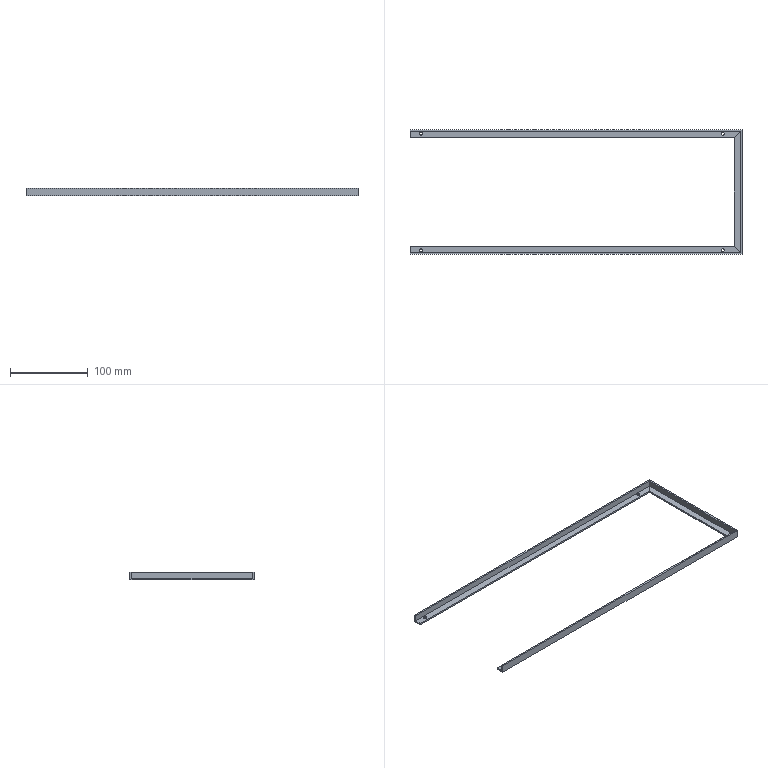Part | STEP file | 1-43.2 | 1 solid | 24 faces | box 427 x 160 x 10 mm | volume 35939 mm3 | plane 20 | cylinder 4 | commonest cylinder face diameters 4 x4
STEP:
#1=CARTESIAN_POINT('',(0.,0.,0.));
#2=DIRECTION('',(0.,0.,1.));
#3=DIRECTION('',(1.,0.,0.));
#4=AXIS2_PLACEMENT_3D('',#1,#2,#3);
#5=CARTESIAN_POINT('',(0.,0.,0.));
#6=VERTEX_POINT('',#5);
#7=CARTESIAN_POINT('',(0.,10.,0.));
#8=VERTEX_POINT('',#7);
#9=CARTESIAN_POINT('',(0.,0.,0.));
#10=DIRECTION('',(0.,1.,0.));
#11=VECTOR('',#10,1.);
#12=LINE('',#9,#11);
#13=CARTESIAN_POINT('',(0.,5.,5.));
#14=DIRECTION('',(1.,0.,0.));
#15=DIRECTION('',(0.,0.,1.));
#16=AXIS2_PLACEMENT_3D('',#13,#14,#15);
#17=PLANE('',#16);
#18=CARTESIAN_POINT('',(-5.,5.));
#19=DIRECTION('',(0.,-1.));
#20=VECTOR('',#19,1.);
#21=LINE('',#18,#20);
#22=(GEOMETRIC_REPRESENTATION_CONTEXT(2)PARAMETRIC_REPRESENTATION_CONTEXT()REPRESENTATION_CONTEXT('',''));
#23=DEFINITIONAL_REPRESENTATION('',(#21),#22);
#24=PCURVE('',#17,#23);
#25=CARTESIAN_POINT('',(213.5,5.,0.));
#26=DIRECTION('',(0.,0.,-1.));
#27=DIRECTION('',(0.,1.,0.));
#28=AXIS2_PLACEMENT_3D('',#25,#26,#27);
#29=PLANE('',#28);
#30=CARTESIAN_POINT('',(-5.,-213.5));
#31=DIRECTION('',(1.,0.));
#32=VECTOR('',#31,1.);
#33=LINE('',#30,#32);
#34=(GEOMETRIC_REPRESENTATION_CONTEXT(2)PARAMETRIC_REPRESENTATION_CONTEXT()REPRESENTATION_CONTEXT('',''));
#35=DEFINITIONAL_REPRESENTATION('',(#33),#34);
#36=PCURVE('',#29,#35);
#37=SURFACE_CURVE('',#12,(#24,#36),.PCURVE_S1.);
#38=EDGE_CURVE('',#6,#8,#37,.T.);
#39=ORIENTED_EDGE('',*,*,#38,.T.);
#40=CARTESIAN_POINT('',(0.,10.,2.));
#41=VERTEX_POINT('',#40);
#42=CARTESIAN_POINT('',(0.,10.,0.));
#43=DIRECTION('',(0.,0.,1.));
#44=VECTOR('',#43,1.);
#45=LINE('',#42,#44);
#46=CARTESIAN_POINT('',(-5.,-5.));
#47=DIRECTION('',(1.,0.));
#48=VECTOR('',#47,1.);
#49=LINE('',#46,#48);
#50=(GEOMETRIC_REPRESENTATION_CONTEXT(2)PARAMETRIC_REPRESENTATION_CONTEXT()REPRESENTATION_CONTEXT('',''));
#51=DEFINITIONAL_REPRESENTATION('',(#49),#50);
#52=PCURVE('',#17,#51);
#53=CARTESIAN_POINT('',(213.5,10.,1.));
#54=DIRECTION('',(0.,1.,0.));
#55=DIRECTION('',(0.,0.,1.));
#56=AXIS2_PLACEMENT_3D('',#53,#54,#55);
#57=PLANE('',#56);
#58=CARTESIAN_POINT('',(-1.,-213.5));
#59=DIRECTION('',(1.,0.));
#60=VECTOR('',#59,1.);
#61=LINE('',#58,#60);
#62=(GEOMETRIC_REPRESENTATION_CONTEXT(2)PARAMETRIC_REPRESENTATION_CONTEXT()REPRESENTATION_CONTEXT('',''));
#63=DEFINITIONAL_REPRESENTATION('',(#61),#62);
#64=PCURVE('',#57,#63);
#65=SURFACE_CURVE('',#45,(#52,#64),.PCURVE_S1.);
#66=EDGE_CURVE('',#8,#41,#65,.T.);
#67=ORIENTED_EDGE('',*,*,#66,.T.);
#68=CARTESIAN_POINT('',(0.,2.,2.));
#69=VERTEX_POINT('',#68);
#70=CARTESIAN_POINT('',(0.,10.,2.));
#71=DIRECTION('',(0.,-1.,0.));
#72=VECTOR('',#71,1.);
#73=LINE('',#70,#72);
#74=CARTESIAN_POINT('',(-3.,-5.));
#75=DIRECTION('',(0.,1.));
#76=VECTOR('',#75,1.);
#77=LINE('',#74,#76);
#78=(GEOMETRIC_REPRESENTATION_CONTEXT(2)PARAMETRIC_REPRESENTATION_CONTEXT()REPRESENTATION_CONTEXT('',''));
#79=DEFINITIONAL_REPRESENTATION('',(#77),#78);
#80=PCURVE('',#17,#79);
#81=CARTESIAN_POINT('',(213.5,6.,2.));
#82=DIRECTION('',(0.,0.,1.));
#83=DIRECTION('',(0.,-1.,0.));
#84=AXIS2_PLACEMENT_3D('',#81,#82,#83);
#85=PLANE('',#84);
#86=CARTESIAN_POINT('',(-4.,-213.5));
#87=DIRECTION('',(1.,0.));
#88=VECTOR('',#87,1.);
#89=LINE('',#86,#88);
#90=(GEOMETRIC_REPRESENTATION_CONTEXT(2)PARAMETRIC_REPRESENTATION_CONTEXT()REPRESENTATION_CONTEXT('',''));
#91=DEFINITIONAL_REPRESENTATION('',(#89),#90);
#92=PCURVE('',#85,#91);
#93=SURFACE_CURVE('',#73,(#80,#92),.PCURVE_S1.);
#94=EDGE_CURVE('',#41,#69,#93,.T.);
#95=ORIENTED_EDGE('',*,*,#94,.T.);
#96=CARTESIAN_POINT('',(0.,2.,10.));
#97=VERTEX_POINT('',#96);
#98=CARTESIAN_POINT('',(0.,2.,2.));
#99=DIRECTION('',(0.,0.,1.));
#100=VECTOR('',#99,1.);
#101=LINE('',#98,#100);
#102=CARTESIAN_POINT('',(-3.,3.));
#103=DIRECTION('',(1.,0.));
#104=VECTOR('',#103,1.);
#105=LINE('',#102,#104);
#106=(GEOMETRIC_REPRESENTATION_CONTEXT(2)PARAMETRIC_REPRESENTATION_CONTEXT()REPRESENTATION_CONTEXT('',''));
#107=DEFINITIONAL_REPRESENTATION('',(#105),#106);
#108=PCURVE('',#17,#107);
#109=CARTESIAN_POINT('',(213.5,2.,6.));
#110=DIRECTION('',(0.,1.,0.));
#111=DIRECTION('',(0.,0.,1.));
#112=AXIS2_PLACEMENT_3D('',#109,#110,#111);
#113=PLANE('',#112);
#114=CARTESIAN_POINT('',(-4.,-213.5));
#115=DIRECTION('',(1.,0.));
#116=VECTOR('',#115,1.);
#117=LINE('',#114,#116);
#118=(GEOMETRIC_REPRESENTATION_CONTEXT(2)PARAMETRIC_REPRESENTATION_CONTEXT()REPRESENTATION_CONTEXT('',''));
#119=DEFINITIONAL_REPRESENTATION('',(#117),#118);
#120=PCURVE('',#113,#119);
#121=SURFACE_CURVE('',#101,(#108,#120),.PCURVE_S1.);
#122=EDGE_CURVE('',#69,#97,#121,.T.);
#123=ORIENTED_EDGE('',*,*,#122,.T.);
#124=CARTESIAN_POINT('',(0.,0.,10.));
#125=VERTEX_POINT('',#124);
#126=CARTESIAN_POINT('',(0.,2.,10.));
#127=DIRECTION('',(0.,-1.,0.));
#128=VECTOR('',#127,1.);
#129=LINE('',#126,#128);
#130=CARTESIAN_POINT('',(5.,3.));
#131=DIRECTION('',(0.,1.));
#132=VECTOR('',#131,1.);
#133=LINE('',#130,#132);
#134=(GEOMETRIC_REPRESENTATION_CONTEXT(2)PARAMETRIC_REPRESENTATION_CONTEXT()REPRESENTATION_CONTEXT('',''));
#135=DEFINITIONAL_REPRESENTATION('',(#133),#134);
#136=PCURVE('',#17,#135);
#137=CARTESIAN_POINT('',(213.5,1.,10.));
#138=DIRECTION('',(0.,0.,1.));
#139=DIRECTION('',(0.,-1.,0.));
#140=AXIS2_PLACEMENT_3D('',#137,#138,#139);
#141=PLANE('',#140);
#142=CARTESIAN_POINT('',(-1.,-213.5));
#143=DIRECTION('',(1.,0.));
#144=VECTOR('',#143,1.);
#145=LINE('',#142,#144);
#146=(GEOMETRIC_REPRESENTATION_CONTEXT(2)PARAMETRIC_REPRESENTATION_CONTEXT()REPRESENTATION_CONTEXT('',''));
#147=DEFINITIONAL_REPRESENTATION('',(#145),#146);
#148=PCURVE('',#141,#147);
#149=SURFACE_CURVE('',#129,(#136,#148),.PCURVE_S1.);
#150=EDGE_CURVE('',#97,#125,#149,.T.);
#151=ORIENTED_EDGE('',*,*,#150,.T.);
#152=CARTESIAN_POINT('',(0.,0.,10.));
#153=DIRECTION('',(0.,0.,-1.));
#154=VECTOR('',#153,1.);
#155=LINE('',#152,#154);
#156=CARTESIAN_POINT('',(5.,5.));
#157=DIRECTION('',(-1.,0.));
#158=VECTOR('',#157,1.);
#159=LINE('',#156,#158);
#160=(GEOMETRIC_REPRESENTATION_CONTEXT(2)PARAMETRIC_REPRESENTATION_CONTEXT()REPRESENTATION_CONTEXT('',''));
#161=DEFINITIONAL_REPRESENTATION('',(#159),#160);
#162=PCURVE('',#17,#161);
#163=CARTESIAN_POINT('',(213.5,0.,5.));
#164=DIRECTION('',(0.,-1.,0.));
#165=DIRECTION('',(0.,0.,-1.));
#166=AXIS2_PLACEMENT_3D('',#163,#164,#165);
#167=PLANE('',#166);
#168=CARTESIAN_POINT('',(-5.,-213.5));
#169=DIRECTION('',(1.,0.));
#170=VECTOR('',#169,1.);
#171=LINE('',#168,#170);
#172=(GEOMETRIC_REPRESENTATION_CONTEXT(2)PARAMETRIC_REPRESENTATION_CONTEXT()REPRESENTATION_CONTEXT('',''));
#173=DEFINITIONAL_REPRESENTATION('',(#171),#172);
#174=PCURVE('',#167,#173);
#175=SURFACE_CURVE('',#155,(#162,#174),.PCURVE_S1.);
#176=EDGE_CURVE('',#125,#6,#175,.T.);
#177=ORIENTED_EDGE('',*,*,#176,.T.);
#178=EDGE_LOOP('',(#39,#67,#95,#123,#151,#177));
#179=FACE_BOUND('',#178,.F.);
#180=ADVANCED_FACE('',(#179),#17,.F.);
#181=CARTESIAN_POINT('',(0.,160.,0.));
#182=VERTEX_POINT('',#181);
#183=CARTESIAN_POINT('',(0.,150.,0.));
#184=VERTEX_POINT('',#183);
#185=CARTESIAN_POINT('',(0.,160.,0.));
#186=DIRECTION('',(0.,-1.,0.));
#187=VECTOR('',#186,1.);
#188=LINE('',#185,#187);
#189=CARTESIAN_POINT('',(0.,155.,5.));
#190=DIRECTION('',(-1.,0.,0.));
#191=DIRECTION('',(0.,0.,1.));
#192=AXIS2_PLACEMENT_3D('',#189,#190,#191);
#193=PLANE('',#192);
#194=CARTESIAN_POINT('',(-5.,5.));
#195=DIRECTION('',(0.,-1.));
#196=VECTOR('',#195,1.);
#197=LINE('',#194,#196);
#198=(GEOMETRIC_REPRESENTATION_CONTEXT(2)PARAMETRIC_REPRESENTATION_CONTEXT()REPRESENTATION_CONTEXT('',''));
#199=DEFINITIONAL_REPRESENTATION('',(#197),#198);
#200=PCURVE('',#193,#199);
#201=CARTESIAN_POINT('',(213.5,155.,0.));
#202=DIRECTION('',(0.,0.,-1.));
#203=DIRECTION('',(0.,-1.,0.));
#204=AXIS2_PLACEMENT_3D('',#201,#202,#203);
#205=PLANE('',#204);
#206=CARTESIAN_POINT('',(-5.,213.5));
#207=DIRECTION('',(1.,0.));
#208=VECTOR('',#207,1.);
#209=LINE('',#206,#208);
#210=(GEOMETRIC_REPRESENTATION_CONTEXT(2)PARAMETRIC_REPRESENTATION_CONTEXT()REPRESENTATION_CONTEXT('',''));
#211=DEFINITIONAL_REPRESENTATION('',(#209),#210);
#212=PCURVE('',#205,#211);
#213=SURFACE_CURVE('',#188,(#200,#212),.PCURVE_S1.);
#214=EDGE_CURVE('',#182,#184,#213,.T.);
#215=ORIENTED_EDGE('',*,*,#214,.T.);
#216=CARTESIAN_POINT('',(0.,150.,2.));
#217=VERTEX_POINT('',#216);
#218=CARTESIAN_POINT('',(0.,150.,0.));
#219=DIRECTION('',(0.,0.,1.));
#220=VECTOR('',#219,1.);
#221=LINE('',#218,#220);
#222=CARTESIAN_POINT('',(-5.,-5.));
#223=DIRECTION('',(1.,0.));
#224=VECTOR('',#223,1.);
#225=LINE('',#222,#224);
#226=(GEOMETRIC_REPRESENTATION_CONTEXT(2)PARAMETRIC_REPRESENTATION_CONTEXT()REPRESENTATION_CONTEXT('',''));
#227=DEFINITIONAL_REPRESENTATION('',(#225),#226);
#228=PCURVE('',#193,#227);
#229=CARTESIAN_POINT('',(213.5,150.,1.));
#230=DIRECTION('',(0.,-1.,0.));
#231=DIRECTION('',(0.,0.,1.));
#232=AXIS2_PLACEMENT_3D('',#229,#230,#231);
#233=PLANE('',#232);
#234=CARTESIAN_POINT('',(-1.,213.5));
#235=DIRECTION('',(1.,0.));
#236=VECTOR('',#235,1.);
#237=LINE('',#234,#236);
#238=(GEOMETRIC_REPRESENTATION_CONTEXT(2)PARAMETRIC_REPRESENTATION_CONTEXT()REPRESENTATION_CONTEXT('',''));
#239=DEFINITIONAL_REPRESENTATION('',(#237),#238);
#240=PCURVE('',#233,#239);
#241=SURFACE_CURVE('',#221,(#228,#240),.PCURVE_S1.);
#242=EDGE_CURVE('',#184,#217,#241,.T.);
#243=ORIENTED_EDGE('',*,*,#242,.T.);
#244=CARTESIAN_POINT('',(0.,158.,2.));
#245=VERTEX_POINT('',#244);
#246=CARTESIAN_POINT('',(0.,150.,2.));
#247=DIRECTION('',(0.,1.,0.));
#248=VECTOR('',#247,1.);
#249=LINE('',#246,#248);
#250=CARTESIAN_POINT('',(-3.,-5.));
#251=DIRECTION('',(0.,1.));
#252=VECTOR('',#251,1.);
#253=LINE('',#250,#252);
#254=(GEOMETRIC_REPRESENTATION_CONTEXT(2)PARAMETRIC_REPRESENTATION_CONTEXT()REPRESENTATION_CONTEXT('',''));
#255=DEFINITIONAL_REPRESENTATION('',(#253),#254);
#256=PCURVE('',#193,#255);
#257=CARTESIAN_POINT('',(213.5,154.,2.));
#258=DIRECTION('',(0.,0.,1.));
#259=DIRECTION('',(0.,1.,0.));
#260=AXIS2_PLACEMENT_3D('',#257,#258,#259);
#261=PLANE('',#260);
#262=CARTESIAN_POINT('',(-4.,213.5));
#263=DIRECTION('',(1.,0.));
#264=VECTOR('',#263,1.);
#265=LINE('',#262,#264);
#266=(GEOMETRIC_REPRESENTATION_CONTEXT(2)PARAMETRIC_REPRESENTATION_CONTEXT()REPRESENTATION_CONTEXT('',''));
#267=DEFINITIONAL_REPRESENTATION('',(#265),#266);
#268=PCURVE('',#261,#267);
#269=SURFACE_CURVE('',#249,(#256,#268),.PCURVE_S1.);
#270=EDGE_CURVE('',#217,#245,#269,.T.);
#271=ORIENTED_EDGE('',*,*,#270,.T.);
#272=CARTESIAN_POINT('',(0.,158.,10.));
#273=VERTEX_POINT('',#272);
#274=CARTESIAN_POINT('',(0.,158.,2.));
#275=DIRECTION('',(0.,0.,1.));
#276=VECTOR('',#275,1.);
#277=LINE('',#274,#276);
#278=CARTESIAN_POINT('',(-3.,3.));
#279=DIRECTION('',(1.,0.));
#280=VECTOR('',#279,1.);
#281=LINE('',#278,#280);
#282=(GEOMETRIC_REPRESENTATION_CONTEXT(2)PARAMETRIC_REPRESENTATION_CONTEXT()REPRESENTATION_CONTEXT('',''));
#283=DEFINITIONAL_REPRESENTATION('',(#281),#282);
#284=PCURVE('',#193,#283);
#285=CARTESIAN_POINT('',(213.5,158.,6.));
#286=DIRECTION('',(0.,-1.,0.));
#287=DIRECTION('',(0.,0.,1.));
#288=AXIS2_PLACEMENT_3D('',#285,#286,#287);
#289=PLANE('',#288);
#290=CARTESIAN_POINT('',(-4.,213.5));
#291=DIRECTION('',(1.,0.));
#292=VECTOR('',#291,1.);
#293=LINE('',#290,#292);
#294=(GEOMETRIC_REPRESENTATION_CONTEXT(2)PARAMETRIC_REPRESENTATION_CONTEXT()REPRESENTATION_CONTEXT('',''));
#295=DEFINITIONAL_REPRESENTATION('',(#293),#294);
#296=PCURVE('',#289,#295);
#297=SURFACE_CURVE('',#277,(#284,#296),.PCURVE_S1.);
#298=EDGE_CURVE('',#245,#273,#297,.T.);
#299=ORIENTED_EDGE('',*,*,#298,.T.);
#300=CARTESIAN_POINT('',(0.,160.,10.));
#301=VERTEX_POINT('',#300);
#302=CARTESIAN_POINT('',(0.,158.,10.));
#303=DIRECTION('',(0.,1.,0.));
#304=VECTOR('',#303,1.);
#305=LINE('',#302,#304);
#306=CARTESIAN_POINT('',(5.,3.));
#307=DIRECTION('',(0.,1.));
#308=VECTOR('',#307,1.);
#309=LINE('',#306,#308);
#310=(GEOMETRIC_REPRESENTATION_CONTEXT(2)PARAMETRIC_REPRESENTATION_CONTEXT()REPRESENTATION_CONTEXT('',''));
#311=DEFINITIONAL_REPRESENTATION('',(#309),#310);
#312=PCURVE('',#193,#311);
#313=CARTESIAN_POINT('',(213.5,159.,10.));
#314=DIRECTION('',(0.,0.,1.));
#315=DIRECTION('',(0.,1.,0.));
#316=AXIS2_PLACEMENT_3D('',#313,#314,#315);
#317=PLANE('',#316);
#318=CARTESIAN_POINT('',(-1.,213.5));
#319=DIRECTION('',(1.,0.));
#320=VECTOR('',#319,1.);
#321=LINE('',#318,#320);
#322=(GEOMETRIC_REPRESENTATION_CONTEXT(2)PARAMETRIC_REPRESENTATION_CONTEXT()REPRESENTATION_CONTEXT('',''));
#323=DEFINITIONAL_REPRESENTATION('',(#321),#322);
#324=PCURVE('',#317,#323);
#325=SURFACE_CURVE('',#305,(#312,#324),.PCURVE_S1.);
#326=EDGE_CURVE('',#273,#301,#325,.T.);
#327=ORIENTED_EDGE('',*,*,#326,.T.);
#328=CARTESIAN_POINT('',(0.,160.,10.));
#329=DIRECTION('',(0.,0.,-1.));
#330=VECTOR('',#329,1.);
#331=LINE('',#328,#330);
#332=CARTESIAN_POINT('',(5.,5.));
#333=DIRECTION('',(-1.,0.));
#334=VECTOR('',#333,1.);
#335=LINE('',#332,#334);
#336=(GEOMETRIC_REPRESENTATION_CONTEXT(2)PARAMETRIC_REPRESENTATION_CONTEXT()REPRESENTATION_CONTEXT('',''));
#337=DEFINITIONAL_REPRESENTATION('',(#335),#336);
#338=PCURVE('',#193,#337);
#339=CARTESIAN_POINT('',(213.5,160.,5.));
#340=DIRECTION('',(0.,1.,0.));
#341=DIRECTION('',(0.,0.,-1.));
#342=AXIS2_PLACEMENT_3D('',#339,#340,#341);
#343=PLANE('',#342);
#344=CARTESIAN_POINT('',(-5.,213.5));
#345=DIRECTION('',(1.,0.));
#346=VECTOR('',#345,1.);
#347=LINE('',#344,#346);
#348=(GEOMETRIC_REPRESENTATION_CONTEXT(2)PARAMETRIC_REPRESENTATION_CONTEXT()REPRESENTATION_CONTEXT('',''));
#349=DEFINITIONAL_REPRESENTATION('',(#347),#348);
#350=PCURVE('',#343,#349);
#351=SURFACE_CURVE('',#331,(#338,#350),.PCURVE_S1.);
#352=EDGE_CURVE('',#301,#182,#351,.T.);
#353=ORIENTED_EDGE('',*,*,#352,.T.);
#354=EDGE_LOOP('',(#215,#243,#271,#299,#327,#353));
#355=FACE_BOUND('',#354,.T.);
#356=ADVANCED_FACE('',(#355),#193,.T.);
#357=CARTESIAN_POINT('',(427.,0.,10.));
#358=VERTEX_POINT('',#357);
#359=CARTESIAN_POINT('',(0.,0.,10.));
#360=DIRECTION('',(1.,0.,0.));
#361=VECTOR('',#360,1.);
#362=LINE('',#359,#361);
#363=CARTESIAN_POINT('',(-5.,-213.5));
#364=DIRECTION('',(0.,1.));
#365=VECTOR('',#364,1.);
#366=LINE('',#363,#365);
#367=(GEOMETRIC_REPRESENTATION_CONTEXT(2)PARAMETRIC_REPRESENTATION_CONTEXT()REPRESENTATION_CONTEXT('',''));
#368=DEFINITIONAL_REPRESENTATION('',(#366),#367);
#369=PCURVE('',#167,#368);
#370=CARTESIAN_POINT('',(1.,-213.5));
#371=DIRECTION('',(0.,1.));
#372=VECTOR('',#371,1.);
#373=LINE('',#370,#372);
#374=(GEOMETRIC_REPRESENTATION_CONTEXT(2)PARAMETRIC_REPRESENTATION_CONTEXT()REPRESENTATION_CONTEXT('',''));
#375=DEFINITIONAL_REPRESENTATION('',(#373),#374);
#376=PCURVE('',#141,#375);
#377=SURFACE_CURVE('',#362,(#369,#376),.PCURVE_S1.);
#378=EDGE_CURVE('',#125,#358,#377,.T.);
#379=ORIENTED_EDGE('',*,*,#378,.F.);
#380=ORIENTED_EDGE('',*,*,#176,.T.);
#381=CARTESIAN_POINT('',(427.,0.,0.));
#382=VERTEX_POINT('',#381);
#383=CARTESIAN_POINT('',(0.,0.,0.));
#384=DIRECTION('',(1.,0.,0.));
#385=VECTOR('',#384,1.);
#386=LINE('',#383,#385);
#387=CARTESIAN_POINT('',(5.,-213.5));
#388=DIRECTION('',(0.,1.));
#389=VECTOR('',#388,1.);
#390=LINE('',#387,#389);
#391=(GEOMETRIC_REPRESENTATION_CONTEXT(2)PARAMETRIC_REPRESENTATION_CONTEXT()REPRESENTATION_CONTEXT('',''));
#392=DEFINITIONAL_REPRESENTATION('',(#390),#391);
#393=PCURVE('',#167,#392);
#394=CARTESIAN_POINT('',(-5.,-213.5));
#395=DIRECTION('',(0.,1.));
#396=VECTOR('',#395,1.);
#397=LINE('',#394,#396);
#398=(GEOMETRIC_REPRESENTATION_CONTEXT(2)PARAMETRIC_REPRESENTATION_CONTEXT()REPRESENTATION_CONTEXT('',''));
#399=DEFINITIONAL_REPRESENTATION('',(#397),#398);
#400=PCURVE('',#29,#399);
#401=SURFACE_CURVE('',#386,(#393,#400),.PCURVE_S1.);
#402=EDGE_CURVE('',#6,#382,#401,.T.);
#403=ORIENTED_EDGE('',*,*,#402,.T.);
#404=CARTESIAN_POINT('',(427.,0.,10.));
#405=DIRECTION('',(0.,0.,-1.));
#406=VECTOR('',#405,1.);
#407=LINE('',#404,#406);
#408=CARTESIAN_POINT('',(-5.,213.5));
#409=DIRECTION('',(1.,0.));
#410=VECTOR('',#409,1.);
#411=LINE('',#408,#410);
#412=(GEOMETRIC_REPRESENTATION_CONTEXT(2)PARAMETRIC_REPRESENTATION_CONTEXT()REPRESENTATION_CONTEXT('',''));
#413=DEFINITIONAL_REPRESENTATION('',(#411),#412);
#414=PCURVE('',#167,#413);
#415=CARTESIAN_POINT('',(427.,80.,5.));
#416=DIRECTION('',(1.,0.,0.));
#417=DIRECTION('',(0.,0.,-1.));
#418=AXIS2_PLACEMENT_3D('',#415,#416,#417);
#419=PLANE('',#418);
#420=CARTESIAN_POINT('',(-5.,-80.));
#421=DIRECTION('',(1.,0.));
#422=VECTOR('',#421,1.);
#423=LINE('',#420,#422);
#424=(GEOMETRIC_REPRESENTATION_CONTEXT(2)PARAMETRIC_REPRESENTATION_CONTEXT()REPRESENTATION_CONTEXT('',''));
#425=DEFINITIONAL_REPRESENTATION('',(#423),#424);
#426=PCURVE('',#419,#425);
#427=SURFACE_CURVE('',#407,(#414,#426),.PCURVE_S1.);
#428=EDGE_CURVE('',#358,#382,#427,.T.);
#429=ORIENTED_EDGE('',*,*,#428,.F.);
#430=EDGE_LOOP('',(#379,#380,#403,#429));
#431=FACE_BOUND('',#430,.T.);
#432=ADVANCED_FACE('',(#431),#167,.T.);
#433=ORIENTED_EDGE('',*,*,#66,.T.);
#434=CARTESIAN_POINT('',(417.,10.,2.));
#435=VERTEX_POINT('',#434);
#436=CARTESIAN_POINT('',(0.,10.,2.));
#437=DIRECTION('',(1.,0.,0.));
#438=VECTOR('',#437,1.);
#439=LINE('',#436,#438);
#440=CARTESIAN_POINT('',(1.,-213.5));
#441=DIRECTION('',(0.,1.));
#442=VECTOR('',#441,1.);
#443=LINE('',#440,#442);
#444=(GEOMETRIC_REPRESENTATION_CONTEXT(2)PARAMETRIC_REPRESENTATION_CONTEXT()REPRESENTATION_CONTEXT('',''));
#445=DEFINITIONAL_REPRESENTATION('',(#443),#444);
#446=PCURVE('',#57,#445);
#447=CARTESIAN_POINT('',(-4.,-213.5));
#448=DIRECTION('',(0.,1.));
#449=VECTOR('',#448,1.);
#450=LINE('',#447,#449);
#451=(GEOMETRIC_REPRESENTATION_CONTEXT(2)PARAMETRIC_REPRESENTATION_CONTEXT()REPRESENTATION_CONTEXT('',''));
#452=DEFINITIONAL_REPRESENTATION('',(#450),#451);
#453=PCURVE('',#85,#452);
#454=SURFACE_CURVE('',#439,(#446,#453),.PCURVE_S1.);
#455=EDGE_CURVE('',#41,#435,#454,.T.);
#456=ORIENTED_EDGE('',*,*,#455,.T.);
#457=CARTESIAN_POINT('',(417.,10.,0.));
#458=VERTEX_POINT('',#457);
#459=CARTESIAN_POINT('',(417.,10.,2.));
#460=DIRECTION('',(0.,0.,-1.));
#461=VECTOR('',#460,1.);
#462=LINE('',#459,#461);
#463=CARTESIAN_POINT('',(1.,203.5));
#464=DIRECTION('',(-1.,0.));
#465=VECTOR('',#464,1.);
#466=LINE('',#463,#465);
#467=(GEOMETRIC_REPRESENTATION_CONTEXT(2)PARAMETRIC_REPRESENTATION_CONTEXT()REPRESENTATION_CONTEXT('',''));
#468=DEFINITIONAL_REPRESENTATION('',(#466),#467);
#469=PCURVE('',#57,#468);
#470=CARTESIAN_POINT('',(417.,80.,1.));
#471=DIRECTION('',(-1.,0.,0.));
#472=DIRECTION('',(0.,0.,1.));
#473=AXIS2_PLACEMENT_3D('',#470,#471,#472);
#474=PLANE('',#473);
#475=CARTESIAN_POINT('',(1.,-70.));
#476=DIRECTION('',(-1.,0.));
#477=VECTOR('',#476,1.);
#478=LINE('',#475,#477);
#479=(GEOMETRIC_REPRESENTATION_CONTEXT(2)PARAMETRIC_REPRESENTATION_CONTEXT()REPRESENTATION_CONTEXT('',''));
#480=DEFINITIONAL_REPRESENTATION('',(#478),#479);
#481=PCURVE('',#474,#480);
#482=SURFACE_CURVE('',#462,(#469,#481),.PCURVE_S1.);
#483=EDGE_CURVE('',#435,#458,#482,.T.);
#484=ORIENTED_EDGE('',*,*,#483,.T.);
#485=CARTESIAN_POINT('',(0.,10.,0.));
#486=DIRECTION('',(1.,0.,0.));
#487=VECTOR('',#486,1.);
#488=LINE('',#485,#487);
#489=CARTESIAN_POINT('',(-1.,-213.5));
#490=DIRECTION('',(0.,1.));
#491=VECTOR('',#490,1.);
#492=LINE('',#489,#491);
#493=(GEOMETRIC_REPRESENTATION_CONTEXT(2)PARAMETRIC_REPRESENTATION_CONTEXT()REPRESENTATION_CONTEXT('',''));
#494=DEFINITIONAL_REPRESENTATION('',(#492),#493);
#495=PCURVE('',#57,#494);
#496=CARTESIAN_POINT('',(5.,-213.5));
#497=DIRECTION('',(0.,1.));
#498=VECTOR('',#497,1.);
#499=LINE('',#496,#498);
#500=(GEOMETRIC_REPRESENTATION_CONTEXT(2)PARAMETRIC_REPRESENTATION_CONTEXT()REPRESENTATION_CONTEXT('',''));
#501=DEFINITIONAL_REPRESENTATION('',(#499),#500);
#502=PCURVE('',#29,#501);
#503=SURFACE_CURVE('',#488,(#495,#502),.PCURVE_S1.);
#504=EDGE_CURVE('',#8,#458,#503,.T.);
#505=ORIENTED_EDGE('',*,*,#504,.F.);
#506=EDGE_LOOP('',(#433,#456,#484,#505));
#507=FACE_BOUND('',#506,.T.);
#508=ADVANCED_FACE('',(#507),#57,.T.);
#509=ORIENTED_EDGE('',*,*,#122,.T.);
#510=CARTESIAN_POINT('',(425.,2.,10.));
#511=VERTEX_POINT('',#510);
#512=CARTESIAN_POINT('',(0.,2.,10.));
#513=DIRECTION('',(1.,0.,0.));
#514=VECTOR('',#513,1.);
#515=LINE('',#512,#514);
#516=CARTESIAN_POINT('',(4.,-213.5));
#517=DIRECTION('',(0.,1.));
#518=VECTOR('',#517,1.);
#519=LINE('',#516,#518);
#520=(GEOMETRIC_REPRESENTATION_CONTEXT(2)PARAMETRIC_REPRESENTATION_CONTEXT()REPRESENTATION_CONTEXT('',''));
#521=DEFINITIONAL_REPRESENTATION('',(#519),#520);
#522=PCURVE('',#113,#521);
#523=CARTESIAN_POINT('',(-1.,-213.5));
#524=DIRECTION('',(0.,1.));
#525=VECTOR('',#524,1.);
#526=LINE('',#523,#525);
#527=(GEOMETRIC_REPRESENTATION_CONTEXT(2)PARAMETRIC_REPRESENTATION_CONTEXT()REPRESENTATION_CONTEXT('',''));
#528=DEFINITIONAL_REPRESENTATION('',(#526),#527);
#529=PCURVE('',#141,#528);
#530=SURFACE_CURVE('',#515,(#522,#529),.PCURVE_S1.);
#531=EDGE_CURVE('',#97,#511,#530,.T.);
#532=ORIENTED_EDGE('',*,*,#531,.T.);
#533=CARTESIAN_POINT('',(425.,2.,2.));
#534=VERTEX_POINT('',#533);
#535=CARTESIAN_POINT('',(425.,2.,10.));
#536=DIRECTION('',(0.,0.,-1.));
#537=VECTOR('',#536,1.);
#538=LINE('',#535,#537);
#539=CARTESIAN_POINT('',(4.,211.5));
#540=DIRECTION('',(-1.,0.));
#541=VECTOR('',#540,1.);
#542=LINE('',#539,#541);
#543=(GEOMETRIC_REPRESENTATION_CONTEXT(2)PARAMETRIC_REPRESENTATION_CONTEXT()REPRESENTATION_CONTEXT('',''));
#544=DEFINITIONAL_REPRESENTATION('',(#542),#543);
#545=PCURVE('',#113,#544);
#546=CARTESIAN_POINT('',(425.,80.,6.));
#547=DIRECTION('',(-1.,0.,0.));
#548=DIRECTION('',(0.,0.,1.));
#549=AXIS2_PLACEMENT_3D('',#546,#547,#548);
#550=PLANE('',#549);
#551=CARTESIAN_POINT('',(4.,-78.));
#552=DIRECTION('',(-1.,0.));
#553=VECTOR('',#552,1.);
#554=LINE('',#551,#553);
#555=(GEOMETRIC_REPRESENTATION_CONTEXT(2)PARAMETRIC_REPRESENTATION_CONTEXT()REPRESENTATION_CONTEXT('',''));
#556=DEFINITIONAL_REPRESENTATION('',(#554),#555);
#557=PCURVE('',#550,#556);
#558=SURFACE_CURVE('',#538,(#545,#557),.PCURVE_S1.);
#559=EDGE_CURVE('',#511,#534,#558,.T.);
#560=ORIENTED_EDGE('',*,*,#559,.T.);
#561=CARTESIAN_POINT('',(0.,2.,2.));
#562=DIRECTION('',(1.,0.,0.));
#563=VECTOR('',#562,1.);
#564=LINE('',#561,#563);
#565=CARTESIAN_POINT('',(-4.,-213.5));
#566=DIRECTION('',(0.,1.));
#567=VECTOR('',#566,1.);
#568=LINE('',#565,#567);
#569=(GEOMETRIC_REPRESENTATION_CONTEXT(2)PARAMETRIC_REPRESENTATION_CONTEXT()REPRESENTATION_CONTEXT('',''));
#570=DEFINITIONAL_REPRESENTATION('',(#568),#569);
#571=PCURVE('',#113,#570);
#572=CARTESIAN_POINT('',(4.,-213.5));
#573=DIRECTION('',(0.,1.));
#574=VECTOR('',#573,1.);
#575=LINE('',#572,#574);
#576=(GEOMETRIC_REPRESENTATION_CONTEXT(2)PARAMETRIC_REPRESENTATION_CONTEXT()REPRESENTATION_CONTEXT('',''));
#577=DEFINITIONAL_REPRESENTATION('',(#575),#576);
#578=PCURVE('',#85,#577);
#579=SURFACE_CURVE('',#564,(#571,#578),.PCURVE_S1.);
#580=EDGE_CURVE('',#69,#534,#579,.T.);
#581=ORIENTED_EDGE('',*,*,#580,.F.);
#582=EDGE_LOOP('',(#509,#532,#560,#581));
#583=FACE_BOUND('',#582,.T.);
#584=ADVANCED_FACE('',(#583),#113,.T.);
#585=ORIENTED_EDGE('',*,*,#150,.T.);
#586=ORIENTED_EDGE('',*,*,#378,.T.);
#587=CARTESIAN_POINT('',(427.,0.,10.));
#588=DIRECTION('',(-0.7071,0.7071,0.));
#589=VECTOR('',#588,1.);
#590=LINE('',#587,#589);
#591=CARTESIAN_POINT('',(1.,213.5));
#592=DIRECTION('',(-0.7071,-0.7071));
#593=VECTOR('',#592,1.);
#594=LINE('',#591,#593);
#595=(GEOMETRIC_REPRESENTATION_CONTEXT(2)PARAMETRIC_REPRESENTATION_CONTEXT()REPRESENTATION_CONTEXT('',''));
#596=DEFINITIONAL_REPRESENTATION('',(#594),#595);
#597=PCURVE('',#141,#596);
#598=CARTESIAN_POINT('',(426.,80.,10.));
#599=DIRECTION('',(0.,0.,1.));
#600=DIRECTION('',(1.,0.,0.));
#601=AXIS2_PLACEMENT_3D('',#598,#599,#600);
#602=PLANE('',#601);
#603=CARTESIAN_POINT('',(1.,-80.));
#604=DIRECTION('',(-0.7071,0.7071));
#605=VECTOR('',#604,1.);
#606=LINE('',#603,#605);
#607=(GEOMETRIC_REPRESENTATION_CONTEXT(2)PARAMETRIC_REPRESENTATION_CONTEXT()REPRESENTATION_CONTEXT('',''));
#608=DEFINITIONAL_REPRESENTATION('',(#606),#607);
#609=PCURVE('',#602,#608);
#610=SURFACE_CURVE('',#590,(#597,#609),.PCURVE_S1.);
#611=EDGE_CURVE('',#358,#511,#610,.T.);
#612=ORIENTED_EDGE('',*,*,#611,.T.);
#613=ORIENTED_EDGE('',*,*,#531,.F.);
#614=EDGE_LOOP('',(#585,#586,#612,#613));
#615=FACE_BOUND('',#614,.T.);
#616=ADVANCED_FACE('',(#615),#141,.T.);
#617=CARTESIAN_POINT('',(427.,160.,10.));
#618=VERTEX_POINT('',#617);
#619=CARTESIAN_POINT('',(427.,0.,10.));
#620=DIRECTION('',(0.,1.,0.));
#621=VECTOR('',#620,1.);
#622=LINE('',#619,#621);
#623=CARTESIAN_POINT('',(-5.,-80.));
#624=DIRECTION('',(0.,1.));
#625=VECTOR('',#624,1.);
#626=LINE('',#623,#625);
#627=(GEOMETRIC_REPRESENTATION_CONTEXT(2)PARAMETRIC_REPRESENTATION_CONTEXT()REPRESENTATION_CONTEXT('',''));
#628=DEFINITIONAL_REPRESENTATION('',(#626),#627);
#629=PCURVE('',#419,#628);
#630=CARTESIAN_POINT('',(1.,-80.));
#631=DIRECTION('',(0.,1.));
#632=VECTOR('',#631,1.);
#633=LINE('',#630,#632);
#634=(GEOMETRIC_REPRESENTATION_CONTEXT(2)PARAMETRIC_REPRESENTATION_CONTEXT()REPRESENTATION_CONTEXT('',''));
#635=DEFINITIONAL_REPRESENTATION('',(#633),#634);
#636=PCURVE('',#602,#635);
#637=SURFACE_CURVE('',#622,(#629,#636),.PCURVE_S1.);
#638=EDGE_CURVE('',#358,#618,#637,.T.);
#639=ORIENTED_EDGE('',*,*,#638,.F.);
#640=ORIENTED_EDGE('',*,*,#428,.T.);
#641=CARTESIAN_POINT('',(427.,160.,0.));
#642=VERTEX_POINT('',#641);
#643=CARTESIAN_POINT('',(427.,0.,0.));
#644=DIRECTION('',(0.,1.,0.));
#645=VECTOR('',#644,1.);
#646=LINE('',#643,#645);
#647=CARTESIAN_POINT('',(5.,-80.));
#648=DIRECTION('',(0.,1.));
#649=VECTOR('',#648,1.);
#650=LINE('',#647,#649);
#651=(GEOMETRIC_REPRESENTATION_CONTEXT(2)PARAMETRIC_REPRESENTATION_CONTEXT()REPRESENTATION_CONTEXT('',''));
#652=DEFINITIONAL_REPRESENTATION('',(#650),#651);
#653=PCURVE('',#419,#652);
#654=CARTESIAN_POINT('',(422.,80.,0.));
#655=DIRECTION('',(0.,0.,-1.));
#656=DIRECTION('',(-1.,0.,0.));
#657=AXIS2_PLACEMENT_3D('',#654,#655,#656);
#658=PLANE('',#657);
#659=CARTESIAN_POINT('',(-5.,-80.));
#660=DIRECTION('',(0.,1.));
#661=VECTOR('',#660,1.);
#662=LINE('',#659,#661);
#663=(GEOMETRIC_REPRESENTATION_CONTEXT(2)PARAMETRIC_REPRESENTATION_CONTEXT()REPRESENTATION_CONTEXT('',''));
#664=DEFINITIONAL_REPRESENTATION('',(#662),#663);
#665=PCURVE('',#658,#664);
#666=SURFACE_CURVE('',#646,(#653,#665),.PCURVE_S1.);
#667=EDGE_CURVE('',#382,#642,#666,.T.);
#668=ORIENTED_EDGE('',*,*,#667,.T.);
#669=CARTESIAN_POINT('',(427.,160.,10.));
#670=DIRECTION('',(0.,0.,-1.));
#671=VECTOR('',#670,1.);
#672=LINE('',#669,#671);
#673=CARTESIAN_POINT('',(-5.,80.));
#674=DIRECTION('',(1.,0.));
#675=VECTOR('',#674,1.);
#676=LINE('',#673,#675);
#677=(GEOMETRIC_REPRESENTATION_CONTEXT(2)PARAMETRIC_REPRESENTATION_CONTEXT()REPRESENTATION_CONTEXT('',''));
#678=DEFINITIONAL_REPRESENTATION('',(#676),#677);
#679=PCURVE('',#419,#678);
#680=CARTESIAN_POINT('',(-5.,-213.5));
#681=DIRECTION('',(1.,0.));
#682=VECTOR('',#681,1.);
#683=LINE('',#680,#682);
#684=(GEOMETRIC_REPRESENTATION_CONTEXT(2)PARAMETRIC_REPRESENTATION_CONTEXT()REPRESENTATION_CONTEXT('',''));
#685=DEFINITIONAL_REPRESENTATION('',(#683),#684);
#686=PCURVE('',#343,#685);
#687=SURFACE_CURVE('',#672,(#679,#686),.PCURVE_S1.);
#688=EDGE_CURVE('',#618,#642,#687,.T.);
#689=ORIENTED_EDGE('',*,*,#688,.F.);
#690=EDGE_LOOP('',(#639,#640,#668,#689));
#691=FACE_BOUND('',#690,.T.);
#692=ADVANCED_FACE('',(#691),#419,.T.);
#693=ORIENTED_EDGE('',*,*,#611,.F.);
#694=ORIENTED_EDGE('',*,*,#638,.T.);
#695=CARTESIAN_POINT('',(425.,158.,10.));
#696=VERTEX_POINT('',#695);
#697=CARTESIAN_POINT('',(427.,160.,10.));
#698=DIRECTION('',(-0.7071,-0.7071,0.));
#699=VECTOR('',#698,1.);
#700=LINE('',#697,#699);
#701=CARTESIAN_POINT('',(1.,80.));
#702=DIRECTION('',(-0.7071,-0.7071));
#703=VECTOR('',#702,1.);
#704=LINE('',#701,#703);
#705=(GEOMETRIC_REPRESENTATION_CONTEXT(2)PARAMETRIC_REPRESENTATION_CONTEXT()REPRESENTATION_CONTEXT('',''));
#706=DEFINITIONAL_REPRESENTATION('',(#704),#705);
#707=PCURVE('',#602,#706);
#708=CARTESIAN_POINT('',(1.,-213.5));
#709=DIRECTION('',(-0.7071,0.7071));
#710=VECTOR('',#709,1.);
#711=LINE('',#708,#710);
#712=(GEOMETRIC_REPRESENTATION_CONTEXT(2)PARAMETRIC_REPRESENTATION_CONTEXT()REPRESENTATION_CONTEXT('',''));
#713=DEFINITIONAL_REPRESENTATION('',(#711),#712);
#714=PCURVE('',#317,#713);
#715=SURFACE_CURVE('',#700,(#707,#714),.PCURVE_S1.);
#716=EDGE_CURVE('',#618,#696,#715,.T.);
#717=ORIENTED_EDGE('',*,*,#716,.T.);
#718=CARTESIAN_POINT('',(425.,2.,10.));
#719=DIRECTION('',(0.,1.,0.));
#720=VECTOR('',#719,1.);
#721=LINE('',#718,#720);
#722=CARTESIAN_POINT('',(-1.,-78.));
#723=DIRECTION('',(0.,1.));
#724=VECTOR('',#723,1.);
#725=LINE('',#722,#724);
#726=(GEOMETRIC_REPRESENTATION_CONTEXT(2)PARAMETRIC_REPRESENTATION_CONTEXT()REPRESENTATION_CONTEXT('',''));
#727=DEFINITIONAL_REPRESENTATION('',(#725),#726);
#728=PCURVE('',#602,#727);
#729=CARTESIAN_POINT('',(4.,-78.));
#730=DIRECTION('',(0.,1.));
#731=VECTOR('',#730,1.);
#732=LINE('',#729,#731);
#733=(GEOMETRIC_REPRESENTATION_CONTEXT(2)PARAMETRIC_REPRESENTATION_CONTEXT()REPRESENTATION_CONTEXT('',''));
#734=DEFINITIONAL_REPRESENTATION('',(#732),#733);
#735=PCURVE('',#550,#734);
#736=SURFACE_CURVE('',#721,(#728,#735),.PCURVE_S1.);
#737=EDGE_CURVE('',#511,#696,#736,.T.);
#738=ORIENTED_EDGE('',*,*,#737,.F.);
#739=EDGE_LOOP('',(#693,#694,#717,#738));
#740=FACE_BOUND('',#739,.T.);
#741=ADVANCED_FACE('',(#740),#602,.T.);
#742=ORIENTED_EDGE('',*,*,#667,.F.);
#743=CARTESIAN_POINT('',(417.,10.,0.));
#744=DIRECTION('',(0.7071,-0.7071,0.));
#745=VECTOR('',#744,1.);
#746=LINE('',#743,#745);
#747=CARTESIAN_POINT('',(5.,-70.));
#748=DIRECTION('',(-0.7071,-0.7071));
#749=VECTOR('',#748,1.);
#750=LINE('',#747,#749);
#751=(GEOMETRIC_REPRESENTATION_CONTEXT(2)PARAMETRIC_REPRESENTATION_CONTEXT()REPRESENTATION_CONTEXT('',''));
#752=DEFINITIONAL_REPRESENTATION('',(#750),#751);
#753=PCURVE('',#658,#752);
#754=CARTESIAN_POINT('',(5.,203.5));
#755=DIRECTION('',(-0.7071,0.7071));
#756=VECTOR('',#755,1.);
#757=LINE('',#754,#756);
#758=(GEOMETRIC_REPRESENTATION_CONTEXT(2)PARAMETRIC_REPRESENTATION_CONTEXT()REPRESENTATION_CONTEXT('',''));
#759=DEFINITIONAL_REPRESENTATION('',(#757),#758);
#760=PCURVE('',#29,#759);
#761=SURFACE_CURVE('',#746,(#753,#760),.PCURVE_S1.);
#762=EDGE_CURVE('',#458,#382,#761,.T.);
#763=ORIENTED_EDGE('',*,*,#762,.F.);
#764=CARTESIAN_POINT('',(417.,150.,0.));
#765=VERTEX_POINT('',#764);
#766=CARTESIAN_POINT('',(417.,10.,0.));
#767=DIRECTION('',(0.,1.,0.));
#768=VECTOR('',#767,1.);
#769=LINE('',#766,#768);
#770=CARTESIAN_POINT('',(5.,-70.));
#771=DIRECTION('',(0.,1.));
#772=VECTOR('',#771,1.);
#773=LINE('',#770,#772);
#774=(GEOMETRIC_REPRESENTATION_CONTEXT(2)PARAMETRIC_REPRESENTATION_CONTEXT()REPRESENTATION_CONTEXT('',''));
#775=DEFINITIONAL_REPRESENTATION('',(#773),#774);
#776=PCURVE('',#658,#775);
#777=CARTESIAN_POINT('',(-1.,-70.));
#778=DIRECTION('',(0.,1.));
#779=VECTOR('',#778,1.);
#780=LINE('',#777,#779);
#781=(GEOMETRIC_REPRESENTATION_CONTEXT(2)PARAMETRIC_REPRESENTATION_CONTEXT()REPRESENTATION_CONTEXT('',''));
#782=DEFINITIONAL_REPRESENTATION('',(#780),#781);
#783=PCURVE('',#474,#782);
#784=SURFACE_CURVE('',#769,(#776,#783),.PCURVE_S1.);
#785=EDGE_CURVE('',#458,#765,#784,.T.);
#786=ORIENTED_EDGE('',*,*,#785,.T.);
#787=CARTESIAN_POINT('',(417.,150.,0.));
#788=DIRECTION('',(0.7071,0.7071,0.));
#789=VECTOR('',#788,1.);
#790=LINE('',#787,#789);
#791=CARTESIAN_POINT('',(5.,70.));
#792=DIRECTION('',(-0.7071,0.7071));
#793=VECTOR('',#792,1.);
#794=LINE('',#791,#793);
#795=(GEOMETRIC_REPRESENTATION_CONTEXT(2)PARAMETRIC_REPRESENTATION_CONTEXT()REPRESENTATION_CONTEXT('',''));
#796=DEFINITIONAL_REPRESENTATION('',(#794),#795);
#797=PCURVE('',#658,#796);
#798=CARTESIAN_POINT('',(5.,-203.5));
#799=DIRECTION('',(-0.7071,-0.7071));
#800=VECTOR('',#799,1.);
#801=LINE('',#798,#800);
#802=(GEOMETRIC_REPRESENTATION_CONTEXT(2)PARAMETRIC_REPRESENTATION_CONTEXT()REPRESENTATION_CONTEXT('',''));
#803=DEFINITIONAL_REPRESENTATION('',(#801),#802);
#804=PCURVE('',#205,#803);
#805=SURFACE_CURVE('',#790,(#797,#804),.PCURVE_S1.);
#806=EDGE_CURVE('',#765,#642,#805,.T.);
#807=ORIENTED_EDGE('',*,*,#806,.T.);
#808=EDGE_LOOP('',(#742,#763,#786,#807));
#809=FACE_BOUND('',#808,.T.);
#810=ADVANCED_FACE('',(#809),#658,.T.);
#811=ORIENTED_EDGE('',*,*,#559,.F.);
#812=ORIENTED_EDGE('',*,*,#737,.T.);
#813=CARTESIAN_POINT('',(425.,158.,2.));
#814=VERTEX_POINT('',#813);
#815=CARTESIAN_POINT('',(425.,158.,10.));
#816=DIRECTION('',(0.,0.,-1.));
#817=VECTOR('',#816,1.);
#818=LINE('',#815,#817);
#819=CARTESIAN_POINT('',(4.,78.));
#820=DIRECTION('',(-1.,0.));
#821=VECTOR('',#820,1.);
#822=LINE('',#819,#821);
#823=(GEOMETRIC_REPRESENTATION_CONTEXT(2)PARAMETRIC_REPRESENTATION_CONTEXT()REPRESENTATION_CONTEXT('',''));
#824=DEFINITIONAL_REPRESENTATION('',(#822),#823);
#825=PCURVE('',#550,#824);
#826=CARTESIAN_POINT('',(4.,-211.5));
#827=DIRECTION('',(-1.,0.));
#828=VECTOR('',#827,1.);
#829=LINE('',#826,#828);
#830=(GEOMETRIC_REPRESENTATION_CONTEXT(2)PARAMETRIC_REPRESENTATION_CONTEXT()REPRESENTATION_CONTEXT('',''));
#831=DEFINITIONAL_REPRESENTATION('',(#829),#830);
#832=PCURVE('',#289,#831);
#833=SURFACE_CURVE('',#818,(#825,#832),.PCURVE_S1.);
#834=EDGE_CURVE('',#696,#814,#833,.T.);
#835=ORIENTED_EDGE('',*,*,#834,.T.);
#836=CARTESIAN_POINT('',(425.,2.,2.));
#837=DIRECTION('',(0.,1.,0.));
#838=VECTOR('',#837,1.);
#839=LINE('',#836,#838);
#840=CARTESIAN_POINT('',(-4.,-78.));
#841=DIRECTION('',(0.,1.));
#842=VECTOR('',#841,1.);
#843=LINE('',#840,#842);
#844=(GEOMETRIC_REPRESENTATION_CONTEXT(2)PARAMETRIC_REPRESENTATION_CONTEXT()REPRESENTATION_CONTEXT('',''));
#845=DEFINITIONAL_REPRESENTATION('',(#843),#844);
#846=PCURVE('',#550,#845);
#847=CARTESIAN_POINT('',(421.,80.,2.));
#848=DIRECTION('',(0.,0.,1.));
#849=DIRECTION('',(1.,0.,0.));
#850=AXIS2_PLACEMENT_3D('',#847,#848,#849);
#851=PLANE('',#850);
#852=CARTESIAN_POINT('',(4.,-78.));
#853=DIRECTION('',(0.,1.));
#854=VECTOR('',#853,1.);
#855=LINE('',#852,#854);
#856=(GEOMETRIC_REPRESENTATION_CONTEXT(2)PARAMETRIC_REPRESENTATION_CONTEXT()REPRESENTATION_CONTEXT('',''));
#857=DEFINITIONAL_REPRESENTATION('',(#855),#856);
#858=PCURVE('',#851,#857);
#859=SURFACE_CURVE('',#839,(#846,#858),.PCURVE_S1.);
#860=EDGE_CURVE('',#534,#814,#859,.T.);
#861=ORIENTED_EDGE('',*,*,#860,.F.);
#862=EDGE_LOOP('',(#811,#812,#835,#861));
#863=FACE_BOUND('',#862,.T.);
#864=ADVANCED_FACE('',(#863),#550,.T.);
#865=ORIENTED_EDGE('',*,*,#483,.F.);
#866=CARTESIAN_POINT('',(417.,150.,2.));
#867=VERTEX_POINT('',#866);
#868=CARTESIAN_POINT('',(417.,10.,2.));
#869=DIRECTION('',(0.,1.,0.));
#870=VECTOR('',#869,1.);
#871=LINE('',#868,#870);
#872=CARTESIAN_POINT('',(1.,-70.));
#873=DIRECTION('',(0.,1.));
#874=VECTOR('',#873,1.);
#875=LINE('',#872,#874);
#876=(GEOMETRIC_REPRESENTATION_CONTEXT(2)PARAMETRIC_REPRESENTATION_CONTEXT()REPRESENTATION_CONTEXT('',''));
#877=DEFINITIONAL_REPRESENTATION('',(#875),#876);
#878=PCURVE('',#474,#877);
#879=CARTESIAN_POINT('',(-4.,-70.));
#880=DIRECTION('',(0.,1.));
#881=VECTOR('',#880,1.);
#882=LINE('',#879,#881);
#883=(GEOMETRIC_REPRESENTATION_CONTEXT(2)PARAMETRIC_REPRESENTATION_CONTEXT()REPRESENTATION_CONTEXT('',''));
#884=DEFINITIONAL_REPRESENTATION('',(#882),#883);
#885=PCURVE('',#851,#884);
#886=SURFACE_CURVE('',#871,(#878,#885),.PCURVE_S1.);
#887=EDGE_CURVE('',#435,#867,#886,.T.);
#888=ORIENTED_EDGE('',*,*,#887,.T.);
#889=CARTESIAN_POINT('',(417.,150.,2.));
#890=DIRECTION('',(0.,0.,-1.));
#891=VECTOR('',#890,1.);
#892=LINE('',#889,#891);
#893=CARTESIAN_POINT('',(1.,70.));
#894=DIRECTION('',(-1.,0.));
#895=VECTOR('',#894,1.);
#896=LINE('',#893,#895);
#897=(GEOMETRIC_REPRESENTATION_CONTEXT(2)PARAMETRIC_REPRESENTATION_CONTEXT()REPRESENTATION_CONTEXT('',''));
#898=DEFINITIONAL_REPRESENTATION('',(#896),#897);
#899=PCURVE('',#474,#898);
#900=CARTESIAN_POINT('',(1.,-203.5));
#901=DIRECTION('',(-1.,0.));
#902=VECTOR('',#901,1.);
#903=LINE('',#900,#902);
#904=(GEOMETRIC_REPRESENTATION_CONTEXT(2)PARAMETRIC_REPRESENTATION_CONTEXT()REPRESENTATION_CONTEXT('',''));
#905=DEFINITIONAL_REPRESENTATION('',(#903),#904);
#906=PCURVE('',#233,#905);
#907=SURFACE_CURVE('',#892,(#899,#906),.PCURVE_S1.);
#908=EDGE_CURVE('',#867,#765,#907,.T.);
#909=ORIENTED_EDGE('',*,*,#908,.T.);
#910=ORIENTED_EDGE('',*,*,#785,.F.);
#911=EDGE_LOOP('',(#865,#888,#909,#910));
#912=FACE_BOUND('',#911,.T.);
#913=ADVANCED_FACE('',(#912),#474,.T.);
#914=CARTESIAN_POINT('',(425.,2.,2.));
#915=DIRECTION('',(-0.7071,0.7071,0.));
#916=VECTOR('',#915,1.);
#917=LINE('',#914,#916);
#918=CARTESIAN_POINT('',(4.,-78.));
#919=DIRECTION('',(-0.7071,0.7071));
#920=VECTOR('',#919,1.);
#921=LINE('',#918,#920);
#922=(GEOMETRIC_REPRESENTATION_CONTEXT(2)PARAMETRIC_REPRESENTATION_CONTEXT()REPRESENTATION_CONTEXT('',''));
#923=DEFINITIONAL_REPRESENTATION('',(#921),#922);
#924=PCURVE('',#851,#923);
#925=CARTESIAN_POINT('',(4.,211.5));
#926=DIRECTION('',(-0.7071,-0.7071));
#927=VECTOR('',#926,1.);
#928=LINE('',#925,#927);
#929=(GEOMETRIC_REPRESENTATION_CONTEXT(2)PARAMETRIC_REPRESENTATION_CONTEXT()REPRESENTATION_CONTEXT('',''));
#930=DEFINITIONAL_REPRESENTATION('',(#928),#929);
#931=PCURVE('',#85,#930);
#932=SURFACE_CURVE('',#917,(#924,#931),.PCURVE_S1.);
#933=EDGE_CURVE('',#534,#435,#932,.T.);
#934=ORIENTED_EDGE('',*,*,#933,.F.);
#935=ORIENTED_EDGE('',*,*,#860,.T.);
#936=CARTESIAN_POINT('',(425.,158.,2.));
#937=DIRECTION('',(-0.7071,-0.7071,0.));
#938=VECTOR('',#937,1.);
#939=LINE('',#936,#938);
#940=CARTESIAN_POINT('',(4.,78.));
#941=DIRECTION('',(-0.7071,-0.7071));
#942=VECTOR('',#941,1.);
#943=LINE('',#940,#942);
#944=(GEOMETRIC_REPRESENTATION_CONTEXT(2)PARAMETRIC_REPRESENTATION_CONTEXT()REPRESENTATION_CONTEXT('',''));
#945=DEFINITIONAL_REPRESENTATION('',(#943),#944);
#946=PCURVE('',#851,#945);
#947=CARTESIAN_POINT('',(4.,-211.5));
#948=DIRECTION('',(-0.7071,0.7071));
#949=VECTOR('',#948,1.);
#950=LINE('',#947,#949);
#951=(GEOMETRIC_REPRESENTATION_CONTEXT(2)PARAMETRIC_REPRESENTATION_CONTEXT()REPRESENTATION_CONTEXT('',''));
#952=DEFINITIONAL_REPRESENTATION('',(#950),#951);
#953=PCURVE('',#261,#952);
#954=SURFACE_CURVE('',#939,(#946,#953),.PCURVE_S1.);
#955=EDGE_CURVE('',#814,#867,#954,.T.);
#956=ORIENTED_EDGE('',*,*,#955,.T.);
#957=ORIENTED_EDGE('',*,*,#887,.F.);
#958=EDGE_LOOP('',(#934,#935,#956,#957));
#959=FACE_BOUND('',#958,.T.);
#960=ADVANCED_FACE('',(#959),#851,.T.);
#961=CARTESIAN_POINT('',(427.,160.,10.));
#962=DIRECTION('',(-1.,0.,0.));
#963=VECTOR('',#962,1.);
#964=LINE('',#961,#963);
#965=CARTESIAN_POINT('',(-5.,-213.5));
#966=DIRECTION('',(0.,1.));
#967=VECTOR('',#966,1.);
#968=LINE('',#965,#967);
#969=(GEOMETRIC_REPRESENTATION_CONTEXT(2)PARAMETRIC_REPRESENTATION_CONTEXT()REPRESENTATION_CONTEXT('',''));
#970=DEFINITIONAL_REPRESENTATION('',(#968),#969);
#971=PCURVE('',#343,#970);
#972=CARTESIAN_POINT('',(1.,-213.5));
#973=DIRECTION('',(0.,1.));
#974=VECTOR('',#973,1.);
#975=LINE('',#972,#974);
#976=(GEOMETRIC_REPRESENTATION_CONTEXT(2)PARAMETRIC_REPRESENTATION_CONTEXT()REPRESENTATION_CONTEXT('',''));
#977=DEFINITIONAL_REPRESENTATION('',(#975),#976);
#978=PCURVE('',#317,#977);
#979=SURFACE_CURVE('',#964,(#971,#978),.PCURVE_S1.);
#980=EDGE_CURVE('',#618,#301,#979,.T.);
#981=ORIENTED_EDGE('',*,*,#980,.F.);
#982=ORIENTED_EDGE('',*,*,#688,.T.);
#983=CARTESIAN_POINT('',(427.,160.,0.));
#984=DIRECTION('',(-1.,0.,0.));
#985=VECTOR('',#984,1.);
#986=LINE('',#983,#985);
#987=CARTESIAN_POINT('',(5.,-213.5));
#988=DIRECTION('',(0.,1.));
#989=VECTOR('',#988,1.);
#990=LINE('',#987,#989);
#991=(GEOMETRIC_REPRESENTATION_CONTEXT(2)PARAMETRIC_REPRESENTATION_CONTEXT()REPRESENTATION_CONTEXT('',''));
#992=DEFINITIONAL_REPRESENTATION('',(#990),#991);
#993=PCURVE('',#343,#992);
#994=CARTESIAN_POINT('',(-5.,-213.5));
#995=DIRECTION('',(0.,1.));
#996=VECTOR('',#995,1.);
#997=LINE('',#994,#996);
#998=(GEOMETRIC_REPRESENTATION_CONTEXT(2)PARAMETRIC_REPRESENTATION_CONTEXT()REPRESENTATION_CONTEXT('',''));
#999=DEFINITIONAL_REPRESENTATION('',(#997),#998);
#1000=PCURVE('',#205,#999);
#1001=SURFACE_CURVE('',#986,(#993,#1000),.PCURVE_S1.);
#1002=EDGE_CURVE('',#642,#182,#1001,.T.);
#1003=ORIENTED_EDGE('',*,*,#1002,.T.);
#1004=ORIENTED_EDGE('',*,*,#352,.F.);
#1005=EDGE_LOOP('',(#981,#982,#1003,#1004));
#1006=FACE_BOUND('',#1005,.T.);
#1007=ADVANCED_FACE('',(#1006),#343,.T.);
#1008=CARTESIAN_POINT('',(425.,158.,10.));
#1009=DIRECTION('',(-1.,0.,0.));
#1010=VECTOR('',#1009,1.);
#1011=LINE('',#1008,#1010);
#1012=CARTESIAN_POINT('',(-1.,-211.5));
#1013=DIRECTION('',(0.,1.));
#1014=VECTOR('',#1013,1.);
#1015=LINE('',#1012,#1014);
#1016=(GEOMETRIC_REPRESENTATION_CONTEXT(2)PARAMETRIC_REPRESENTATION_CONTEXT()REPRESENTATION_CONTEXT('',''));
#1017=DEFINITIONAL_REPRESENTATION('',(#1015),#1016);
#1018=PCURVE('',#317,#1017);
#1019=CARTESIAN_POINT('',(4.,-211.5));
#1020=DIRECTION('',(0.,1.));
#1021=VECTOR('',#1020,1.);
#1022=LINE('',#1019,#1021);
#1023=(GEOMETRIC_REPRESENTATION_CONTEXT(2)PARAMETRIC_REPRESENTATION_CONTEXT()REPRESENTATION_CONTEXT('',''));
#1024=DEFINITIONAL_REPRESENTATION('',(#1022),#1023);
#1025=PCURVE('',#289,#1024);
#1026=SURFACE_CURVE('',#1011,(#1018,#1025),.PCURVE_S1.);
#1027=EDGE_CURVE('',#696,#273,#1026,.T.);
#1028=ORIENTED_EDGE('',*,*,#1027,.F.);
#1029=ORIENTED_EDGE('',*,*,#716,.F.);
#1030=ORIENTED_EDGE('',*,*,#980,.T.);
#1031=ORIENTED_EDGE('',*,*,#326,.F.);
#1032=EDGE_LOOP('',(#1028,#1029,#1030,#1031));
#1033=FACE_BOUND('',#1032,.T.);
#1034=ADVANCED_FACE('',(#1033),#317,.T.);
#1035=CARTESIAN_POINT('',(425.,158.,2.));
#1036=DIRECTION('',(-1.,0.,0.));
#1037=VECTOR('',#1036,1.);
#1038=LINE('',#1035,#1037);
#1039=CARTESIAN_POINT('',(-4.,-211.5));
#1040=DIRECTION('',(0.,1.));
#1041=VECTOR('',#1040,1.);
#1042=LINE('',#1039,#1041);
#1043=(GEOMETRIC_REPRESENTATION_CONTEXT(2)PARAMETRIC_REPRESENTATION_CONTEXT()REPRESENTATION_CONTEXT('',''));
#1044=DEFINITIONAL_REPRESENTATION('',(#1042),#1043);
#1045=PCURVE('',#289,#1044);
#1046=CARTESIAN_POINT('',(4.,-211.5));
#1047=DIRECTION('',(0.,1.));
#1048=VECTOR('',#1047,1.);
#1049=LINE('',#1046,#1048);
#1050=(GEOMETRIC_REPRESENTATION_CONTEXT(2)PARAMETRIC_REPRESENTATION_CONTEXT()REPRESENTATION_CONTEXT('',''));
#1051=DEFINITIONAL_REPRESENTATION('',(#1049),#1050);
#1052=PCURVE('',#261,#1051);
#1053=SURFACE_CURVE('',#1038,(#1045,#1052),.PCURVE_S1.);
#1054=EDGE_CURVE('',#814,#245,#1053,.T.);
#1055=ORIENTED_EDGE('',*,*,#1054,.F.);
#1056=ORIENTED_EDGE('',*,*,#834,.F.);
#1057=ORIENTED_EDGE('',*,*,#1027,.T.);
#1058=ORIENTED_EDGE('',*,*,#298,.F.);
#1059=EDGE_LOOP('',(#1055,#1056,#1057,#1058));
#1060=FACE_BOUND('',#1059,.T.);
#1061=ADVANCED_FACE('',(#1060),#289,.T.);
#1062=CARTESIAN_POINT('',(417.,150.,0.));
#1063=DIRECTION('',(-1.,0.,0.));
#1064=VECTOR('',#1063,1.);
#1065=LINE('',#1062,#1064);
#1066=CARTESIAN_POINT('',(-1.,-203.5));
#1067=DIRECTION('',(0.,1.));
#1068=VECTOR('',#1067,1.);
#1069=LINE('',#1066,#1068);
#1070=(GEOMETRIC_REPRESENTATION_CONTEXT(2)PARAMETRIC_REPRESENTATION_CONTEXT()REPRESENTATION_CONTEXT('',''));
#1071=DEFINITIONAL_REPRESENTATION('',(#1069),#1070);
#1072=PCURVE('',#233,#1071);
#1073=CARTESIAN_POINT('',(5.,-203.5));
#1074=DIRECTION('',(0.,1.));
#1075=VECTOR('',#1074,1.);
#1076=LINE('',#1073,#1075);
#1077=(GEOMETRIC_REPRESENTATION_CONTEXT(2)PARAMETRIC_REPRESENTATION_CONTEXT()REPRESENTATION_CONTEXT('',''));
#1078=DEFINITIONAL_REPRESENTATION('',(#1076),#1077);
#1079=PCURVE('',#205,#1078);
#1080=SURFACE_CURVE('',#1065,(#1072,#1079),.PCURVE_S1.);
#1081=EDGE_CURVE('',#765,#184,#1080,.T.);
#1082=ORIENTED_EDGE('',*,*,#1081,.F.);
#1083=ORIENTED_EDGE('',*,*,#908,.F.);
#1084=CARTESIAN_POINT('',(417.,150.,2.));
#1085=DIRECTION('',(-1.,0.,0.));
#1086=VECTOR('',#1085,1.);
#1087=LINE('',#1084,#1086);
#1088=CARTESIAN_POINT('',(1.,-203.5));
#1089=DIRECTION('',(0.,1.));
#1090=VECTOR('',#1089,1.);
#1091=LINE('',#1088,#1090);
#1092=(GEOMETRIC_REPRESENTATION_CONTEXT(2)PARAMETRIC_REPRESENTATION_CONTEXT()REPRESENTATION_CONTEXT('',''));
#1093=DEFINITIONAL_REPRESENTATION('',(#1091),#1092);
#1094=PCURVE('',#233,#1093);
#1095=CARTESIAN_POINT('',(-4.,-203.5));
#1096=DIRECTION('',(0.,1.));
#1097=VECTOR('',#1096,1.);
#1098=LINE('',#1095,#1097);
#1099=(GEOMETRIC_REPRESENTATION_CONTEXT(2)PARAMETRIC_REPRESENTATION_CONTEXT()REPRESENTATION_CONTEXT('',''));
#1100=DEFINITIONAL_REPRESENTATION('',(#1098),#1099);
#1101=PCURVE('',#261,#1100);
#1102=SURFACE_CURVE('',#1087,(#1094,#1101),.PCURVE_S1.);
#1103=EDGE_CURVE('',#867,#217,#1102,.T.);
#1104=ORIENTED_EDGE('',*,*,#1103,.T.);
#1105=ORIENTED_EDGE('',*,*,#242,.F.);
#1106=EDGE_LOOP('',(#1082,#1083,#1104,#1105));
#1107=FACE_BOUND('',#1106,.T.);
#1108=ADVANCED_FACE('',(#1107),#233,.T.);
#1109=ORIENTED_EDGE('',*,*,#402,.F.);
#1110=ORIENTED_EDGE('',*,*,#38,.T.);
#1111=ORIENTED_EDGE('',*,*,#504,.T.);
#1112=ORIENTED_EDGE('',*,*,#762,.T.);
#1113=EDGE_LOOP('',(#1109,#1110,#1111,#1112));
#1114=FACE_BOUND('',#1113,.T.);
#1115=CARTESIAN_POINT('',(16.,5.,0.));
#1116=VERTEX_POINT('',#1115);
#1117=CARTESIAN_POINT('',(14.,5.,0.));
#1118=DIRECTION('',(0.,0.,-1.));
#1119=DIRECTION('',(1.,0.,0.));
#1120=AXIS2_PLACEMENT_3D('',#1117,#1118,#1119);
#1121=CIRCLE('',#1120,2.);
#1122=CARTESIAN_POINT('',(0.,-199.5));
#1123=DIRECTION('',(0.,1.));
#1124=AXIS2_PLACEMENT_2D('',#1122,#1123);
#1125=CIRCLE('',#1124,2.);
#1126=(GEOMETRIC_REPRESENTATION_CONTEXT(2)PARAMETRIC_REPRESENTATION_CONTEXT()REPRESENTATION_CONTEXT('',''));
#1127=DEFINITIONAL_REPRESENTATION('',(#1125),#1126);
#1128=PCURVE('',#29,#1127);
#1129=CARTESIAN_POINT('',(14.,5.,-7.5));
#1130=DIRECTION('',(0.,0.,1.));
#1131=DIRECTION('',(1.,0.,0.));
#1132=AXIS2_PLACEMENT_3D('',#1129,#1130,#1131);
#1133=CYLINDRICAL_SURFACE('',#1132,2.);
#1134=CARTESIAN_POINT('',(6.283,7.5));
#1135=DIRECTION('',(-1.,0.));
#1136=VECTOR('',#1135,1.);
#1137=LINE('',#1134,#1136);
#1138=(GEOMETRIC_REPRESENTATION_CONTEXT(2)PARAMETRIC_REPRESENTATION_CONTEXT()REPRESENTATION_CONTEXT('',''));
#1139=DEFINITIONAL_REPRESENTATION('',(#1137),#1138);
#1140=PCURVE('',#1133,#1139);
#1141=SURFACE_CURVE('',#1121,(#1128,#1140),.PCURVE_S1.);
#1142=EDGE_CURVE('',#1116,#1116,#1141,.T.);
#1143=ORIENTED_EDGE('',*,*,#1142,.F.);
#1144=EDGE_LOOP('',(#1143));
#1145=FACE_BOUND('',#1144,.T.);
#1146=CARTESIAN_POINT('',(404.,5.,0.));
#1147=VERTEX_POINT('',#1146);
#1148=CARTESIAN_POINT('',(402.,5.,0.));
#1149=DIRECTION('',(0.,0.,-1.));
#1150=DIRECTION('',(1.,0.,0.));
#1151=AXIS2_PLACEMENT_3D('',#1148,#1149,#1150);
#1152=CIRCLE('',#1151,2.);
#1153=CARTESIAN_POINT('',(0.,188.5));
#1154=DIRECTION('',(0.,1.));
#1155=AXIS2_PLACEMENT_2D('',#1153,#1154);
#1156=CIRCLE('',#1155,2.);
#1157=(GEOMETRIC_REPRESENTATION_CONTEXT(2)PARAMETRIC_REPRESENTATION_CONTEXT()REPRESENTATION_CONTEXT('',''));
#1158=DEFINITIONAL_REPRESENTATION('',(#1156),#1157);
#1159=PCURVE('',#29,#1158);
#1160=CARTESIAN_POINT('',(402.,5.,-7.5));
#1161=DIRECTION('',(0.,0.,1.));
#1162=DIRECTION('',(1.,0.,0.));
#1163=AXIS2_PLACEMENT_3D('',#1160,#1161,#1162);
#1164=CYLINDRICAL_SURFACE('',#1163,2.);
#1165=CARTESIAN_POINT('',(6.283,7.5));
#1166=DIRECTION('',(-1.,0.));
#1167=VECTOR('',#1166,1.);
#1168=LINE('',#1165,#1167);
#1169=(GEOMETRIC_REPRESENTATION_CONTEXT(2)PARAMETRIC_REPRESENTATION_CONTEXT()REPRESENTATION_CONTEXT('',''));
#1170=DEFINITIONAL_REPRESENTATION('',(#1168),#1169);
#1171=PCURVE('',#1164,#1170);
#1172=SURFACE_CURVE('',#1152,(#1159,#1171),.PCURVE_S1.);
#1173=EDGE_CURVE('',#1147,#1147,#1172,.T.);
#1174=ORIENTED_EDGE('',*,*,#1173,.F.);
#1175=EDGE_LOOP('',(#1174));
#1176=FACE_BOUND('',#1175,.T.);
#1177=ADVANCED_FACE('',(#1114,#1145,#1176),#29,.T.);
#1178=ORIENTED_EDGE('',*,*,#94,.T.);
#1179=ORIENTED_EDGE('',*,*,#580,.T.);
#1180=ORIENTED_EDGE('',*,*,#933,.T.);
#1181=ORIENTED_EDGE('',*,*,#455,.F.);
#1182=EDGE_LOOP('',(#1178,#1179,#1180,#1181));
#1183=FACE_BOUND('',#1182,.T.);
#1184=CARTESIAN_POINT('',(16.,5.,2.));
#1185=VERTEX_POINT('',#1184);
#1186=CARTESIAN_POINT('',(14.,5.,2.));
#1187=DIRECTION('',(0.,0.,1.));
#1188=DIRECTION('',(1.,0.,0.));
#1189=AXIS2_PLACEMENT_3D('',#1186,#1187,#1188);
#1190=CIRCLE('',#1189,2.);
#1191=CARTESIAN_POINT('',(1.,-199.5));
#1192=DIRECTION('',(0.,1.));
#1193=AXIS2_PLACEMENT_2D('',#1191,#1192);
#1194=CIRCLE('',#1193,2.);
#1195=(GEOMETRIC_REPRESENTATION_CONTEXT(2)PARAMETRIC_REPRESENTATION_CONTEXT()REPRESENTATION_CONTEXT('',''));
#1196=DEFINITIONAL_REPRESENTATION('',(#1194),#1195);
#1197=PCURVE('',#85,#1196);
#1198=CARTESIAN_POINT('',(0.,9.5));
#1199=DIRECTION('',(1.,0.));
#1200=VECTOR('',#1199,1.);
#1201=LINE('',#1198,#1200);
#1202=(GEOMETRIC_REPRESENTATION_CONTEXT(2)PARAMETRIC_REPRESENTATION_CONTEXT()REPRESENTATION_CONTEXT('',''));
#1203=DEFINITIONAL_REPRESENTATION('',(#1201),#1202);
#1204=PCURVE('',#1133,#1203);
#1205=SURFACE_CURVE('',#1190,(#1197,#1204),.PCURVE_S1.);
#1206=EDGE_CURVE('',#1185,#1185,#1205,.T.);
#1207=ORIENTED_EDGE('',*,*,#1206,.F.);
#1208=EDGE_LOOP('',(#1207));
#1209=FACE_BOUND('',#1208,.T.);
#1210=CARTESIAN_POINT('',(404.,5.,2.));
#1211=VERTEX_POINT('',#1210);
#1212=CARTESIAN_POINT('',(402.,5.,2.));
#1213=DIRECTION('',(0.,0.,1.));
#1214=DIRECTION('',(1.,0.,0.));
#1215=AXIS2_PLACEMENT_3D('',#1212,#1213,#1214);
#1216=CIRCLE('',#1215,2.);
#1217=CARTESIAN_POINT('',(1.,188.5));
#1218=DIRECTION('',(0.,1.));
#1219=AXIS2_PLACEMENT_2D('',#1217,#1218);
#1220=CIRCLE('',#1219,2.);
#1221=(GEOMETRIC_REPRESENTATION_CONTEXT(2)PARAMETRIC_REPRESENTATION_CONTEXT()REPRESENTATION_CONTEXT('',''));
#1222=DEFINITIONAL_REPRESENTATION('',(#1220),#1221);
#1223=PCURVE('',#85,#1222);
#1224=CARTESIAN_POINT('',(0.,9.5));
#1225=DIRECTION('',(1.,0.));
#1226=VECTOR('',#1225,1.);
#1227=LINE('',#1224,#1226);
#1228=(GEOMETRIC_REPRESENTATION_CONTEXT(2)PARAMETRIC_REPRESENTATION_CONTEXT()REPRESENTATION_CONTEXT('',''));
#1229=DEFINITIONAL_REPRESENTATION('',(#1227),#1228);
#1230=PCURVE('',#1164,#1229);
#1231=SURFACE_CURVE('',#1216,(#1223,#1230),.PCURVE_S1.);
#1232=EDGE_CURVE('',#1211,#1211,#1231,.T.);
#1233=ORIENTED_EDGE('',*,*,#1232,.F.);
#1234=EDGE_LOOP('',(#1233));
#1235=FACE_BOUND('',#1234,.T.);
#1236=ADVANCED_FACE('',(#1183,#1209,#1235),#85,.T.);
#1237=ORIENTED_EDGE('',*,*,#1002,.F.);
#1238=ORIENTED_EDGE('',*,*,#806,.F.);
#1239=ORIENTED_EDGE('',*,*,#1081,.T.);
#1240=ORIENTED_EDGE('',*,*,#214,.F.);
#1241=EDGE_LOOP('',(#1237,#1238,#1239,#1240));
#1242=FACE_BOUND('',#1241,.T.);
#1243=CARTESIAN_POINT('',(16.,155.,0.));
#1244=VERTEX_POINT('',#1243);
#1245=CARTESIAN_POINT('',(14.,155.,0.));
#1246=DIRECTION('',(0.,0.,-1.));
#1247=DIRECTION('',(1.,0.,0.));
#1248=AXIS2_PLACEMENT_3D('',#1245,#1246,#1247);
#1249=CIRCLE('',#1248,2.);
#1250=CARTESIAN_POINT('',(0.,199.5));
#1251=DIRECTION('',(0.,-1.));
#1252=AXIS2_PLACEMENT_2D('',#1250,#1251);
#1253=CIRCLE('',#1252,2.);
#1254=(GEOMETRIC_REPRESENTATION_CONTEXT(2)PARAMETRIC_REPRESENTATION_CONTEXT()REPRESENTATION_CONTEXT('',''));
#1255=DEFINITIONAL_REPRESENTATION('',(#1253),#1254);
#1256=PCURVE('',#205,#1255);
#1257=CARTESIAN_POINT('',(14.,155.,-7.5));
#1258=DIRECTION('',(0.,0.,1.));
#1259=DIRECTION('',(1.,0.,0.));
#1260=AXIS2_PLACEMENT_3D('',#1257,#1258,#1259);
#1261=CYLINDRICAL_SURFACE('',#1260,2.);
#1262=CARTESIAN_POINT('',(6.283,7.5));
#1263=DIRECTION('',(-1.,0.));
#1264=VECTOR('',#1263,1.);
#1265=LINE('',#1262,#1264);
#1266=(GEOMETRIC_REPRESENTATION_CONTEXT(2)PARAMETRIC_REPRESENTATION_CONTEXT()REPRESENTATION_CONTEXT('',''));
#1267=DEFINITIONAL_REPRESENTATION('',(#1265),#1266);
#1268=PCURVE('',#1261,#1267);
#1269=SURFACE_CURVE('',#1249,(#1256,#1268),.PCURVE_S1.);
#1270=EDGE_CURVE('',#1244,#1244,#1269,.T.);
#1271=ORIENTED_EDGE('',*,*,#1270,.F.);
#1272=EDGE_LOOP('',(#1271));
#1273=FACE_BOUND('',#1272,.T.);
#1274=CARTESIAN_POINT('',(404.,155.,0.));
#1275=VERTEX_POINT('',#1274);
#1276=CARTESIAN_POINT('',(402.,155.,0.));
#1277=DIRECTION('',(0.,0.,-1.));
#1278=DIRECTION('',(1.,0.,0.));
#1279=AXIS2_PLACEMENT_3D('',#1276,#1277,#1278);
#1280=CIRCLE('',#1279,2.);
#1281=CARTESIAN_POINT('',(0.,-188.5));
#1282=DIRECTION('',(0.,-1.));
#1283=AXIS2_PLACEMENT_2D('',#1281,#1282);
#1284=CIRCLE('',#1283,2.);
#1285=(GEOMETRIC_REPRESENTATION_CONTEXT(2)PARAMETRIC_REPRESENTATION_CONTEXT()REPRESENTATION_CONTEXT('',''));
#1286=DEFINITIONAL_REPRESENTATION('',(#1284),#1285);
#1287=PCURVE('',#205,#1286);
#1288=CARTESIAN_POINT('',(402.,155.,-7.5));
#1289=DIRECTION('',(0.,0.,1.));
#1290=DIRECTION('',(1.,0.,0.));
#1291=AXIS2_PLACEMENT_3D('',#1288,#1289,#1290);
#1292=CYLINDRICAL_SURFACE('',#1291,2.);
#1293=CARTESIAN_POINT('',(6.283,7.5));
#1294=DIRECTION('',(-1.,0.));
#1295=VECTOR('',#1294,1.);
#1296=LINE('',#1293,#1295);
#1297=(GEOMETRIC_REPRESENTATION_CONTEXT(2)PARAMETRIC_REPRESENTATION_CONTEXT()REPRESENTATION_CONTEXT('',''));
#1298=DEFINITIONAL_REPRESENTATION('',(#1296),#1297);
#1299=PCURVE('',#1292,#1298);
#1300=SURFACE_CURVE('',#1280,(#1287,#1299),.PCURVE_S1.);
#1301=EDGE_CURVE('',#1275,#1275,#1300,.T.);
#1302=ORIENTED_EDGE('',*,*,#1301,.F.);
#1303=EDGE_LOOP('',(#1302));
#1304=FACE_BOUND('',#1303,.T.);
#1305=ADVANCED_FACE('',(#1242,#1273,#1304),#205,.T.);
#1306=ORIENTED_EDGE('',*,*,#1103,.F.);
#1307=ORIENTED_EDGE('',*,*,#955,.F.);
#1308=ORIENTED_EDGE('',*,*,#1054,.T.);
#1309=ORIENTED_EDGE('',*,*,#270,.F.);
#1310=EDGE_LOOP('',(#1306,#1307,#1308,#1309));
#1311=FACE_BOUND('',#1310,.T.);
#1312=CARTESIAN_POINT('',(16.,155.,2.));
#1313=VERTEX_POINT('',#1312);
#1314=CARTESIAN_POINT('',(14.,155.,2.));
#1315=DIRECTION('',(0.,0.,1.));
#1316=DIRECTION('',(1.,0.,0.));
#1317=AXIS2_PLACEMENT_3D('',#1314,#1315,#1316);
#1318=CIRCLE('',#1317,2.);
#1319=CARTESIAN_POINT('',(1.,199.5));
#1320=DIRECTION('',(0.,-1.));
#1321=AXIS2_PLACEMENT_2D('',#1319,#1320);
#1322=CIRCLE('',#1321,2.);
#1323=(GEOMETRIC_REPRESENTATION_CONTEXT(2)PARAMETRIC_REPRESENTATION_CONTEXT()REPRESENTATION_CONTEXT('',''));
#1324=DEFINITIONAL_REPRESENTATION('',(#1322),#1323);
#1325=PCURVE('',#261,#1324);
#1326=CARTESIAN_POINT('',(0.,9.5));
#1327=DIRECTION('',(1.,0.));
#1328=VECTOR('',#1327,1.);
#1329=LINE('',#1326,#1328);
#1330=(GEOMETRIC_REPRESENTATION_CONTEXT(2)PARAMETRIC_REPRESENTATION_CONTEXT()REPRESENTATION_CONTEXT('',''));
#1331=DEFINITIONAL_REPRESENTATION('',(#1329),#1330);
#1332=PCURVE('',#1261,#1331);
#1333=SURFACE_CURVE('',#1318,(#1325,#1332),.PCURVE_S1.);
#1334=EDGE_CURVE('',#1313,#1313,#1333,.T.);
#1335=ORIENTED_EDGE('',*,*,#1334,.F.);
#1336=EDGE_LOOP('',(#1335));
#1337=FACE_BOUND('',#1336,.T.);
#1338=CARTESIAN_POINT('',(404.,155.,2.));
#1339=VERTEX_POINT('',#1338);
#1340=CARTESIAN_POINT('',(402.,155.,2.));
#1341=DIRECTION('',(0.,0.,1.));
#1342=DIRECTION('',(1.,0.,0.));
#1343=AXIS2_PLACEMENT_3D('',#1340,#1341,#1342);
#1344=CIRCLE('',#1343,2.);
#1345=CARTESIAN_POINT('',(1.,-188.5));
#1346=DIRECTION('',(0.,-1.));
#1347=AXIS2_PLACEMENT_2D('',#1345,#1346);
#1348=CIRCLE('',#1347,2.);
#1349=(GEOMETRIC_REPRESENTATION_CONTEXT(2)PARAMETRIC_REPRESENTATION_CONTEXT()REPRESENTATION_CONTEXT('',''));
#1350=DEFINITIONAL_REPRESENTATION('',(#1348),#1349);
#1351=PCURVE('',#261,#1350);
#1352=CARTESIAN_POINT('',(0.,9.5));
#1353=DIRECTION('',(1.,0.));
#1354=VECTOR('',#1353,1.);
#1355=LINE('',#1352,#1354);
#1356=(GEOMETRIC_REPRESENTATION_CONTEXT(2)PARAMETRIC_REPRESENTATION_CONTEXT()REPRESENTATION_CONTEXT('',''));
#1357=DEFINITIONAL_REPRESENTATION('',(#1355),#1356);
#1358=PCURVE('',#1292,#1357);
#1359=SURFACE_CURVE('',#1344,(#1351,#1358),.PCURVE_S1.);
#1360=EDGE_CURVE('',#1339,#1339,#1359,.T.);
#1361=ORIENTED_EDGE('',*,*,#1360,.F.);
#1362=EDGE_LOOP('',(#1361));
#1363=FACE_BOUND('',#1362,.T.);
#1364=ADVANCED_FACE('',(#1311,#1337,#1363),#261,.T.);
#1365=CARTESIAN_POINT('',(16.,5.,0.));
#1366=DIRECTION('',(0.,0.,1.));
#1367=VECTOR('',#1366,1.);
#1368=LINE('',#1365,#1367);
#1369=CARTESIAN_POINT('',(0.,7.5));
#1370=DIRECTION('',(0.,1.));
#1371=VECTOR('',#1370,1.);
#1372=LINE('',#1369,#1371);
#1373=(GEOMETRIC_REPRESENTATION_CONTEXT(2)PARAMETRIC_REPRESENTATION_CONTEXT()REPRESENTATION_CONTEXT('',''));
#1374=DEFINITIONAL_REPRESENTATION('',(#1372),#1373);
#1375=PCURVE('',#1133,#1374);
#1376=CARTESIAN_POINT('',(6.283,7.5));
#1377=DIRECTION('',(0.,1.));
#1378=VECTOR('',#1377,1.);
#1379=LINE('',#1376,#1378);
#1380=(GEOMETRIC_REPRESENTATION_CONTEXT(2)PARAMETRIC_REPRESENTATION_CONTEXT()REPRESENTATION_CONTEXT('',''));
#1381=DEFINITIONAL_REPRESENTATION('',(#1379),#1380);
#1382=PCURVE('',#1133,#1381);
#1383=SEAM_CURVE('',#1368,(#1375,#1382),.PCURVE_S1.);
#1384=EDGE_CURVE('',#1116,#1185,#1383,.T.);
#1385=ORIENTED_EDGE('',*,*,#1384,.F.);
#1386=ORIENTED_EDGE('',*,*,#1142,.F.);
#1387=ORIENTED_EDGE('',*,*,#1384,.T.);
#1388=ORIENTED_EDGE('',*,*,#1206,.F.);
#1389=EDGE_LOOP('',(#1385,#1386,#1387,#1388));
#1390=FACE_BOUND('',#1389,.F.);
#1391=ADVANCED_FACE('',(#1390),#1133,.F.);
#1392=CARTESIAN_POINT('',(404.,5.,0.));
#1393=DIRECTION('',(0.,0.,1.));
#1394=VECTOR('',#1393,1.);
#1395=LINE('',#1392,#1394);
#1396=CARTESIAN_POINT('',(0.,7.5));
#1397=DIRECTION('',(0.,1.));
#1398=VECTOR('',#1397,1.);
#1399=LINE('',#1396,#1398);
#1400=(GEOMETRIC_REPRESENTATION_CONTEXT(2)PARAMETRIC_REPRESENTATION_CONTEXT()REPRESENTATION_CONTEXT('',''));
#1401=DEFINITIONAL_REPRESENTATION('',(#1399),#1400);
#1402=PCURVE('',#1164,#1401);
#1403=CARTESIAN_POINT('',(6.283,7.5));
#1404=DIRECTION('',(0.,1.));
#1405=VECTOR('',#1404,1.);
#1406=LINE('',#1403,#1405);
#1407=(GEOMETRIC_REPRESENTATION_CONTEXT(2)PARAMETRIC_REPRESENTATION_CONTEXT()REPRESENTATION_CONTEXT('',''));
#1408=DEFINITIONAL_REPRESENTATION('',(#1406),#1407);
#1409=PCURVE('',#1164,#1408);
#1410=SEAM_CURVE('',#1395,(#1402,#1409),.PCURVE_S1.);
#1411=EDGE_CURVE('',#1147,#1211,#1410,.T.);
#1412=ORIENTED_EDGE('',*,*,#1411,.F.);
#1413=ORIENTED_EDGE('',*,*,#1173,.F.);
#1414=ORIENTED_EDGE('',*,*,#1411,.T.);
#1415=ORIENTED_EDGE('',*,*,#1232,.F.);
#1416=EDGE_LOOP('',(#1412,#1413,#1414,#1415));
#1417=FACE_BOUND('',#1416,.F.);
#1418=ADVANCED_FACE('',(#1417),#1164,.F.);
#1419=CARTESIAN_POINT('',(16.,155.,0.));
#1420=DIRECTION('',(0.,0.,1.));
#1421=VECTOR('',#1420,1.);
#1422=LINE('',#1419,#1421);
#1423=CARTESIAN_POINT('',(6.283,7.5));
#1424=DIRECTION('',(0.,1.));
#1425=VECTOR('',#1424,1.);
#1426=LINE('',#1423,#1425);
#1427=(GEOMETRIC_REPRESENTATION_CONTEXT(2)PARAMETRIC_REPRESENTATION_CONTEXT()REPRESENTATION_CONTEXT('',''));
#1428=DEFINITIONAL_REPRESENTATION('',(#1426),#1427);
#1429=PCURVE('',#1261,#1428);
#1430=CARTESIAN_POINT('',(0.,7.5));
#1431=DIRECTION('',(0.,1.));
#1432=VECTOR('',#1431,1.);
#1433=LINE('',#1430,#1432);
#1434=(GEOMETRIC_REPRESENTATION_CONTEXT(2)PARAMETRIC_REPRESENTATION_CONTEXT()REPRESENTATION_CONTEXT('',''));
#1435=DEFINITIONAL_REPRESENTATION('',(#1433),#1434);
#1436=PCURVE('',#1261,#1435);
#1437=SEAM_CURVE('',#1422,(#1429,#1436),.PCURVE_S1.);
#1438=EDGE_CURVE('',#1244,#1313,#1437,.T.);
#1439=ORIENTED_EDGE('',*,*,#1438,.T.);
#1440=ORIENTED_EDGE('',*,*,#1334,.F.);
#1441=ORIENTED_EDGE('',*,*,#1438,.F.);
#1442=ORIENTED_EDGE('',*,*,#1270,.F.);
#1443=EDGE_LOOP('',(#1439,#1440,#1441,#1442));
#1444=FACE_BOUND('',#1443,.F.);
#1445=ADVANCED_FACE('',(#1444),#1261,.F.);
#1446=CARTESIAN_POINT('',(404.,155.,0.));
#1447=DIRECTION('',(0.,0.,1.));
#1448=VECTOR('',#1447,1.);
#1449=LINE('',#1446,#1448);
#1450=CARTESIAN_POINT('',(6.283,7.5));
#1451=DIRECTION('',(0.,1.));
#1452=VECTOR('',#1451,1.);
#1453=LINE('',#1450,#1452);
#1454=(GEOMETRIC_REPRESENTATION_CONTEXT(2)PARAMETRIC_REPRESENTATION_CONTEXT()REPRESENTATION_CONTEXT('',''));
#1455=DEFINITIONAL_REPRESENTATION('',(#1453),#1454);
#1456=PCURVE('',#1292,#1455);
#1457=CARTESIAN_POINT('',(0.,7.5));
#1458=DIRECTION('',(0.,1.));
#1459=VECTOR('',#1458,1.);
#1460=LINE('',#1457,#1459);
#1461=(GEOMETRIC_REPRESENTATION_CONTEXT(2)PARAMETRIC_REPRESENTATION_CONTEXT()REPRESENTATION_CONTEXT('',''));
#1462=DEFINITIONAL_REPRESENTATION('',(#1460),#1461);
#1463=PCURVE('',#1292,#1462);
#1464=SEAM_CURVE('',#1449,(#1456,#1463),.PCURVE_S1.);
#1465=EDGE_CURVE('',#1275,#1339,#1464,.T.);
#1466=ORIENTED_EDGE('',*,*,#1465,.T.);
#1467=ORIENTED_EDGE('',*,*,#1360,.F.);
#1468=ORIENTED_EDGE('',*,*,#1465,.F.);
#1469=ORIENTED_EDGE('',*,*,#1301,.F.);
#1470=EDGE_LOOP('',(#1466,#1467,#1468,#1469));
#1471=FACE_BOUND('',#1470,.F.);
#1472=ADVANCED_FACE('',(#1471),#1292,.F.);
#1473=CLOSED_SHELL('',(#180,#356,#432,#508,#584,#616,#692,#741,#810,#864,#913,#960,#1007,#1034,#1061,#1108,#1177,#1236,#1305,#1364,#1391,#1418,#1445,#1472));
#1474=MANIFOLD_SOLID_BREP('',#1473);
#1475=(LENGTH_UNIT()NAMED_UNIT(*)SI_UNIT(.MILLI.,.METRE.));
#1476=UNCERTAINTY_MEASURE_WITH_UNIT(LENGTH_MEASURE(0.0000001),#1475,'','');
#1477=(NAMED_UNIT(*)PLANE_ANGLE_UNIT()SI_UNIT($,.RADIAN.));
#1478=(NAMED_UNIT(*)SI_UNIT($,.STERADIAN.)SOLID_ANGLE_UNIT());
#1479=(GEOMETRIC_REPRESENTATION_CONTEXT(3)GLOBAL_UNCERTAINTY_ASSIGNED_CONTEXT((#1476))GLOBAL_UNIT_ASSIGNED_CONTEXT((#1475,#1477,#1478))REPRESENTATION_CONTEXT('',''));
#1480=ADVANCED_BREP_SHAPE_REPRESENTATION('',(#4,#1474),#1479);